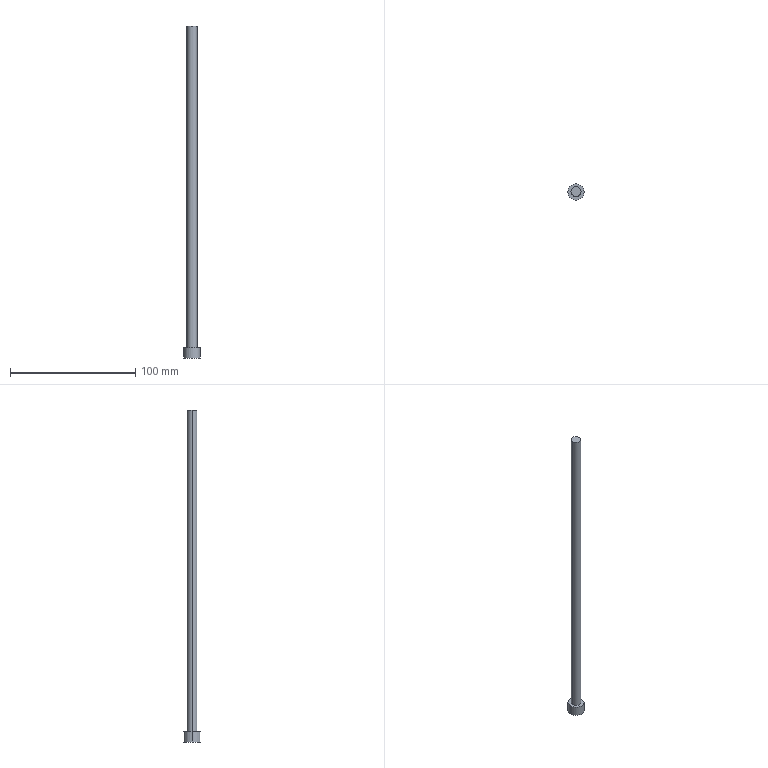Part | Creo | 1 solid | 7 faces | box 13 x 13 x 265.581 mm | volume 14009 mm3 | cylinder 4 | plane 3 | commonest cylinder face diameters 8 x2 13 x2
STEP:
#1=CARTESIAN_POINT('',(0.,0.,0.));
#2=DIRECTION('',(0.,0.,1.));
#3=DIRECTION('',(1.,0.,0.));
#4=AXIS2_PLACEMENT_3D('',#1,#2,#3);
#5=CARTESIAN_POINT('',(5.,69.,-217.5));
#6=VERTEX_POINT('',#5);
#7=CARTESIAN_POINT('',(13.,69.,-217.5));
#8=VERTEX_POINT('',#7);
#9=CARTESIAN_POINT('',(9.,69.,-217.5));
#10=DIRECTION('',(0.,0.,-1.));
#11=DIRECTION('',(-1.,0.,0.));
#12=AXIS2_PLACEMENT_3D('',#9,#10,#11);
#13=CIRCLE('',#12,4.);
#14=EDGE_CURVE('',#6,#8,#13,.T.);
#15=ORIENTED_EDGE('',*,*,#14,.T.);
#16=CARTESIAN_POINT('',(13.,69.,40.081));
#17=VERTEX_POINT('',#16);
#18=CARTESIAN_POINT('',(13.,69.,40.081));
#19=DIRECTION('',(0.,0.,-1.));
#20=VECTOR('',#19,257.581);
#21=LINE('',#18,#20);
#22=EDGE_CURVE('',#17,#8,#21,.T.);
#23=ORIENTED_EDGE('',*,*,#22,.F.);
#24=CARTESIAN_POINT('',(5.,69.,40.081));
#25=VERTEX_POINT('',#24);
#26=CARTESIAN_POINT('',(9.,69.,40.081));
#27=DIRECTION('',(0.,0.,1.));
#28=DIRECTION('',(1.,0.,0.));
#29=AXIS2_PLACEMENT_3D('',#26,#27,#28);
#30=CIRCLE('',#29,4.);
#31=EDGE_CURVE('',#17,#25,#30,.T.);
#32=ORIENTED_EDGE('',*,*,#31,.T.);
#33=CARTESIAN_POINT('',(5.,69.,40.081));
#34=DIRECTION('',(0.,0.,-1.));
#35=VECTOR('',#34,257.581);
#36=LINE('',#33,#35);
#37=EDGE_CURVE('',#25,#6,#36,.T.);
#38=ORIENTED_EDGE('',*,*,#37,.T.);
#39=EDGE_LOOP('',(#15,#23,#32,#38));
#40=FACE_OUTER_BOUND('',#39,.F.);
#41=CARTESIAN_POINT('',(9.,69.,125.91));
#42=DIRECTION('',(0.,0.,-1.));
#43=DIRECTION('',(-1.,0.,0.));
#44=AXIS2_PLACEMENT_3D('',#41,#42,#43);
#45=CYLINDRICAL_SURFACE('',#44,4.);
#46=ADVANCED_FACE('',(#40),#45,.T.);
#47=CARTESIAN_POINT('',(2.5,69.,-217.5));
#48=VERTEX_POINT('',#47);
#49=CARTESIAN_POINT('',(15.5,69.,-217.5));
#50=VERTEX_POINT('',#49);
#51=CARTESIAN_POINT('',(9.,69.,-217.5));
#52=DIRECTION('',(0.,0.,1.));
#53=DIRECTION('',(-1.,0.,0.));
#54=AXIS2_PLACEMENT_3D('',#51,#52,#53);
#55=CIRCLE('',#54,6.5);
#56=EDGE_CURVE('',#48,#50,#55,.T.);
#57=ORIENTED_EDGE('',*,*,#56,.F.);
#58=CARTESIAN_POINT('',(9.,69.,-217.5));
#59=DIRECTION('',(0.,0.,1.));
#60=DIRECTION('',(1.,0.,0.));
#61=AXIS2_PLACEMENT_3D('',#58,#59,#60);
#62=CIRCLE('',#61,6.5);
#63=EDGE_CURVE('',#50,#48,#62,.T.);
#64=ORIENTED_EDGE('',*,*,#63,.F.);
#65=EDGE_LOOP('',(#57,#64));
#66=FACE_OUTER_BOUND('',#65,.F.);
#67=ORIENTED_EDGE('',*,*,#14,.F.);
#68=CARTESIAN_POINT('',(9.,69.,-217.5));
#69=DIRECTION('',(0.,0.,-1.));
#70=DIRECTION('',(1.,0.,0.));
#71=AXIS2_PLACEMENT_3D('',#68,#69,#70);
#72=CIRCLE('',#71,4.);
#73=EDGE_CURVE('',#8,#6,#72,.T.);
#74=ORIENTED_EDGE('',*,*,#73,.F.);
#75=EDGE_LOOP('',(#67,#74));
#76=FACE_BOUND('',#75,.F.);
#77=CARTESIAN_POINT('',(46.5,-0.5,-217.5));
#78=DIRECTION('',(0.,0.,-1.));
#79=DIRECTION('',(-1.,0.,0.));
#80=AXIS2_PLACEMENT_3D('',#77,#78,#79);
#81=PLANE('',#80);
#82=ADVANCED_FACE('',(#66,#76),#81,.F.);
#83=CARTESIAN_POINT('',(15.5,69.,-225.5));
#84=VERTEX_POINT('',#83);
#85=CARTESIAN_POINT('',(2.5,69.,-225.5));
#86=VERTEX_POINT('',#85);
#87=CARTESIAN_POINT('',(9.,69.,-225.5));
#88=DIRECTION('',(0.,0.,-1.));
#89=DIRECTION('',(1.,0.,0.));
#90=AXIS2_PLACEMENT_3D('',#87,#88,#89);
#91=CIRCLE('',#90,6.5);
#92=EDGE_CURVE('',#84,#86,#91,.T.);
#93=ORIENTED_EDGE('',*,*,#92,.T.);
#94=CARTESIAN_POINT('',(2.5,69.,-225.5));
#95=DIRECTION('',(0.,0.,1.));
#96=VECTOR('',#95,8.);
#97=LINE('',#94,#96);
#98=EDGE_CURVE('',#86,#48,#97,.T.);
#99=ORIENTED_EDGE('',*,*,#98,.T.);
#100=ORIENTED_EDGE('',*,*,#56,.T.);
#101=CARTESIAN_POINT('',(15.5,69.,-225.5));
#102=DIRECTION('',(0.,0.,1.));
#103=VECTOR('',#102,8.);
#104=LINE('',#101,#103);
#105=EDGE_CURVE('',#84,#50,#104,.T.);
#106=ORIENTED_EDGE('',*,*,#105,.F.);
#107=EDGE_LOOP('',(#93,#99,#100,#106));
#108=FACE_OUTER_BOUND('',#107,.F.);
#109=CARTESIAN_POINT('',(9.,69.,-225.5));
#110=DIRECTION('',(0.,0.,1.));
#111=DIRECTION('',(1.,0.,0.));
#112=AXIS2_PLACEMENT_3D('',#109,#110,#111);
#113=CYLINDRICAL_SURFACE('',#112,6.5);
#114=ADVANCED_FACE('',(#108),#113,.T.);
#115=CARTESIAN_POINT('',(9.,69.,-225.5));
#116=DIRECTION('',(0.,0.,-1.));
#117=DIRECTION('',(-1.,0.,0.));
#118=AXIS2_PLACEMENT_3D('',#115,#116,#117);
#119=CIRCLE('',#118,6.5);
#120=EDGE_CURVE('',#86,#84,#119,.T.);
#121=ORIENTED_EDGE('',*,*,#120,.F.);
#122=ORIENTED_EDGE('',*,*,#92,.F.);
#123=EDGE_LOOP('',(#121,#122));
#124=FACE_OUTER_BOUND('',#123,.F.);
#125=CARTESIAN_POINT('',(46.5,-0.5,-225.5));
#126=DIRECTION('',(0.,0.,-1.));
#127=DIRECTION('',(-1.,0.,0.));
#128=AXIS2_PLACEMENT_3D('',#125,#126,#127);
#129=PLANE('',#128);
#130=ADVANCED_FACE('',(#124),#129,.T.);
#131=ORIENTED_EDGE('',*,*,#120,.T.);
#132=ORIENTED_EDGE('',*,*,#105,.T.);
#133=ORIENTED_EDGE('',*,*,#63,.T.);
#134=ORIENTED_EDGE('',*,*,#98,.F.);
#135=EDGE_LOOP('',(#131,#132,#133,#134));
#136=FACE_OUTER_BOUND('',#135,.F.);
#137=CARTESIAN_POINT('',(9.,69.,-225.5));
#138=DIRECTION('',(0.,0.,1.));
#139=DIRECTION('',(1.,0.,0.));
#140=AXIS2_PLACEMENT_3D('',#137,#138,#139);
#141=CYLINDRICAL_SURFACE('',#140,6.5);
#142=ADVANCED_FACE('',(#136),#141,.T.);
#143=ORIENTED_EDGE('',*,*,#73,.T.);
#144=ORIENTED_EDGE('',*,*,#37,.F.);
#145=CARTESIAN_POINT('',(9.,69.,40.081));
#146=DIRECTION('',(0.,0.,1.));
#147=DIRECTION('',(-1.,0.,0.));
#148=AXIS2_PLACEMENT_3D('',#145,#146,#147);
#149=CIRCLE('',#148,4.);
#150=EDGE_CURVE('',#25,#17,#149,.T.);
#151=ORIENTED_EDGE('',*,*,#150,.T.);
#152=ORIENTED_EDGE('',*,*,#22,.T.);
#153=EDGE_LOOP('',(#143,#144,#151,#152));
#154=FACE_OUTER_BOUND('',#153,.F.);
#155=CARTESIAN_POINT('',(9.,69.,125.91));
#156=DIRECTION('',(0.,0.,-1.));
#157=DIRECTION('',(-1.,0.,0.));
#158=AXIS2_PLACEMENT_3D('',#155,#156,#157);
#159=CYLINDRICAL_SURFACE('',#158,4.);
#160=ADVANCED_FACE('',(#154),#159,.T.);
#161=ORIENTED_EDGE('',*,*,#31,.F.);
#162=ORIENTED_EDGE('',*,*,#150,.F.);
#163=EDGE_LOOP('',(#161,#162));
#164=FACE_OUTER_BOUND('',#163,.F.);
#165=CARTESIAN_POINT('',(34.847,1.336,40.081));
#166=DIRECTION('',(0.,0.,1.));
#167=DIRECTION('',(1.,0.,0.));
#168=AXIS2_PLACEMENT_3D('',#165,#166,#167);
#169=PLANE('',#168);
#170=ADVANCED_FACE('',(#164),#169,.T.);
#171=CLOSED_SHELL('',(#46,#82,#114,#130,#142,#160,#170));
#172=MANIFOLD_SOLID_BREP('',#171);
#173=(LENGTH_UNIT()NAMED_UNIT(*)SI_UNIT(.MILLI.,.METRE.));
#174=UNCERTAINTY_MEASURE_WITH_UNIT(LENGTH_MEASURE(0.02662),#173,'','');
#175=(NAMED_UNIT(*)PLANE_ANGLE_UNIT()SI_UNIT($,.RADIAN.));
#176=PLANE_ANGLE_MEASURE_WITH_UNIT(PLANE_ANGLE_MEASURE(0.01745),#175);
#177=(CONVERSION_BASED_UNIT('DEGREE',#176)NAMED_UNIT(*)PLANE_ANGLE_UNIT());
#178=(NAMED_UNIT(*)SI_UNIT($,.STERADIAN.)SOLID_ANGLE_UNIT());
#179=(GEOMETRIC_REPRESENTATION_CONTEXT(3)GLOBAL_UNCERTAINTY_ASSIGNED_CONTEXT((#174))GLOBAL_UNIT_ASSIGNED_CONTEXT((#173,#177,#178))REPRESENTATION_CONTEXT('',''));
#180=ADVANCED_BREP_SHAPE_REPRESENTATION('',(#4,#172),#179);